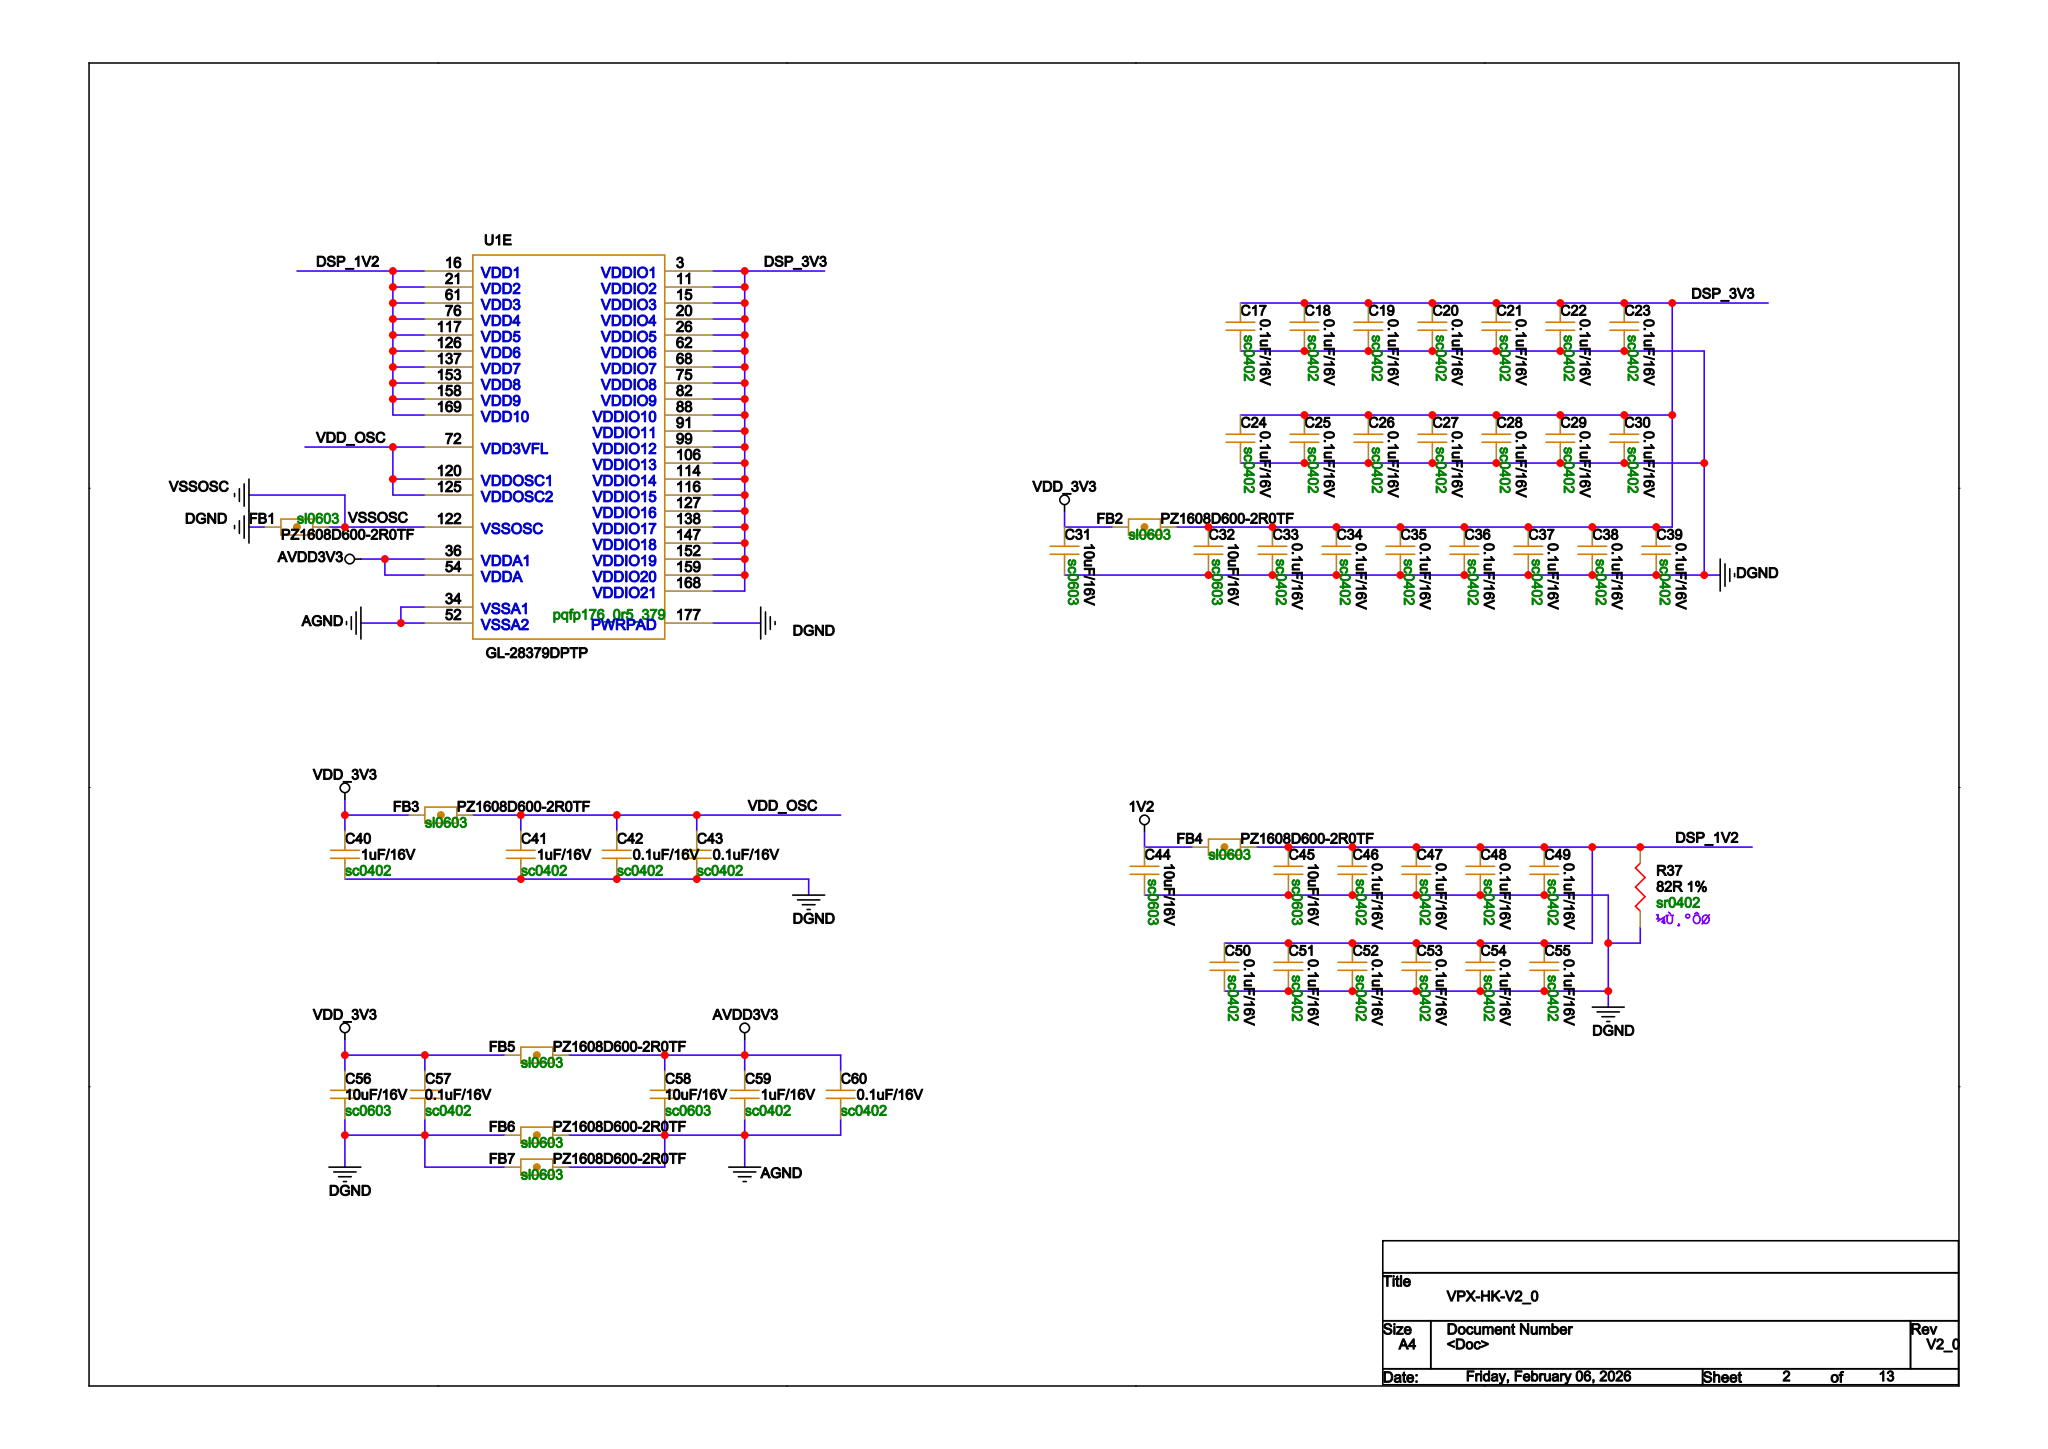Circuit board | Cadence Allegro | 598 parts | 541 nets | one sheet of the schematic
Parts on this sheet (reference | value | footprint):
C40 | 1uF/16V | SC0402
C41 | 1uF/16V | SC0402
C42 | 0.1uF/16V | SC0402
C43 | 0.1uF/16V | SC0402
C56 | 10uF/16V | SC0603
C57 | 0.1uF/16V | SC0402
C58 | 10uF/16V | SC0603
C59 | 1uF/16V | SC0402
C60 | 0.1uF/16V | SC0402
FB1 | PZ1608D600-2R0TF | SL0603
FB2 | PZ1608D600-2R0TF | SL0603
FB3 | PZ1608D600-2R0TF | SL0603
FB4 | PZ1608D600-2R0TF | SL0603
FB5 | PZ1608D600-2R0TF | SL0603
FB6 | PZ1608D600-2R0TF | SL0603
FB7 | PZ1608D600-2R0TF | SL0603
R37 | 82R 1% | SR0402
U1 | GL-28379DPTP | PQFP176_0R5_379
Nets of these parts (net: part-pin ...):
1V2: FB4-1
DGND: C40-2 C41-2 C42-2 C43-2 C56-2 C57-2 FB1-1 FB6-1 FB7-1 R37-2 U1-177
VDD_3V3: C40-1 C56-1 C57-1 FB2-1 FB3-1 FB5-1
AGND: C58-2 C59-2 C60-2 FB6-2 FB7-2 U1-34 U1-52
VSSOSC: FB1-2 U1-122
DSP_3V3: FB2-2 U1-3 U1-11 U1-15 U1-20 U1-26 U1-62 U1-68 U1-75 U1-82 U1-88 U1-91 U1-99 U1-106 U1-114 U1-116 U1-127 U1-138 U1-147 U1-152 U1-159 U1-168
VDD_OSC: C41-1 C42-1 C43-1 FB3-2 U1-72 U1-120 U1-125
DSP_1V2: FB4-2 R37-1 U1-16 U1-21 U1-61 U1-76 U1-117 U1-126 U1-137 U1-153 U1-158 U1-169
AVDD3V3: C58-1 C59-1 C60-1 FB5-2 U1-36 U1-54